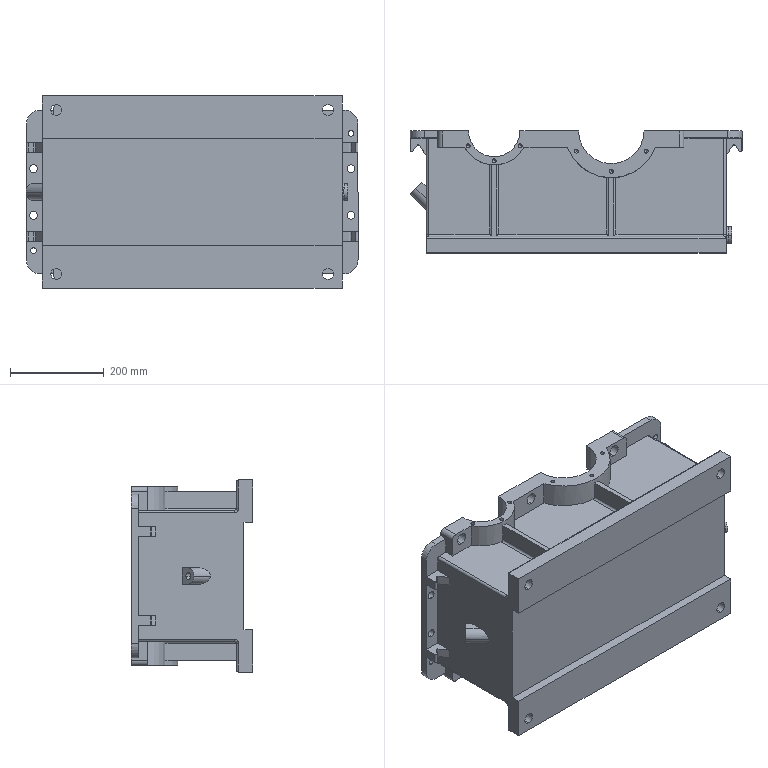Part | SolidWorks | features ICE 11, MirrorPattern 5, Fillet 4, HoleWzd 4, CirPattern 3, Rib 2, Extrusion 1, LPattern 1 | 1 solid | 253 faces | box 708.739 x 260 x 410 mm | volume 11835781 mm3 | cylinder 129 | plane 87 | cone 24 | torus 11 | spline 2 | commonest cylinder face diameters 10 x29 8.5 x24 25 x12 5.8 x8 17 x8 23 x8